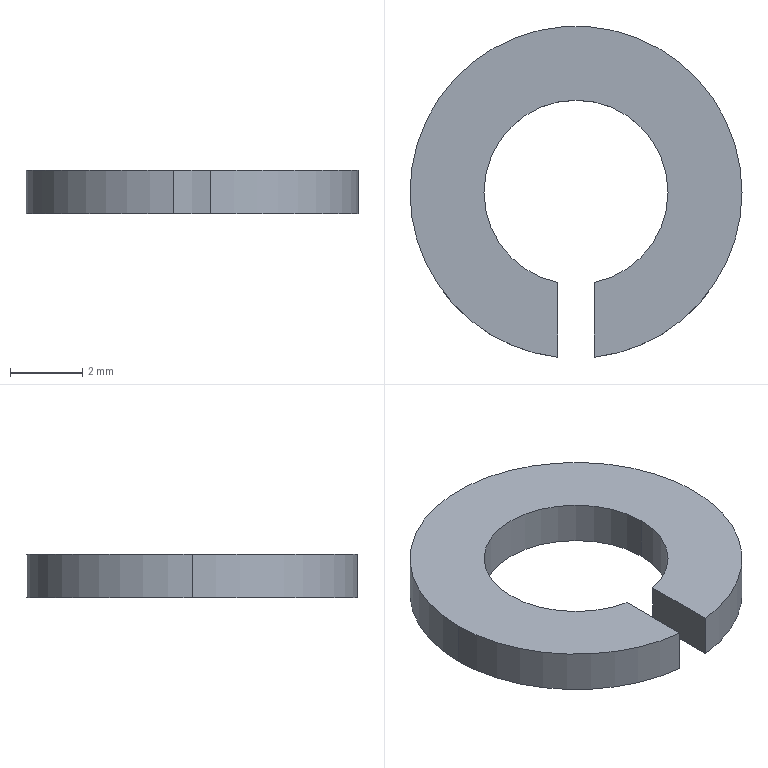Part | NX | features BREP 1 | 1 solid | 10 faces | box 9.2 x 9.173 x 1.2 mm | volume 52.789 mm3 | cylinder 6 | plane 4 | commonest cylinder face diameters 5.1 x3 9.2 x3
STEP:
#1=CARTESIAN_POINT('',(2.55,0.,1.2));
#2=VERTEX_POINT('',#1);
#3=CARTESIAN_POINT('',(0.5,-2.5,1.2));
#4=VERTEX_POINT('',#3);
#5=CARTESIAN_POINT('',(0.,0.,1.2));
#6=DIRECTION('',(0.,0.,-1.));
#7=DIRECTION('',(1.,0.,0.));
#8=AXIS2_PLACEMENT_3D('',#5,#6,#7);
#9=CIRCLE('',#8,2.55);
#10=EDGE_CURVE('',#2,#4,#9,.T.);
#11=ORIENTED_EDGE('',*,*,#10,.F.);
#12=CARTESIAN_POINT('',(2.55,0.,0.));
#13=VERTEX_POINT('',#12);
#14=CARTESIAN_POINT('',(2.55,0.,1.2));
#15=DIRECTION('',(0.,0.,-1.));
#16=VECTOR('',#15,1000.);
#17=LINE('',#14,#16);
#18=EDGE_CURVE('',#2,#13,#17,.T.);
#19=ORIENTED_EDGE('',*,*,#18,.T.);
#20=CARTESIAN_POINT('',(0.5,-2.5,0.));
#21=VERTEX_POINT('',#20);
#22=CARTESIAN_POINT('',(0.,0.,0.));
#23=DIRECTION('',(0.,0.,-1.));
#24=DIRECTION('',(1.,0.,0.));
#25=AXIS2_PLACEMENT_3D('',#22,#23,#24);
#26=CIRCLE('',#25,2.55);
#27=EDGE_CURVE('',#13,#21,#26,.T.);
#28=ORIENTED_EDGE('',*,*,#27,.T.);
#29=CARTESIAN_POINT('',(0.5,-2.5,1.2));
#30=DIRECTION('',(0.,0.,-1.));
#31=VECTOR('',#30,1000.);
#32=LINE('',#29,#31);
#33=EDGE_CURVE('',#4,#21,#32,.T.);
#34=ORIENTED_EDGE('',*,*,#33,.F.);
#35=EDGE_LOOP('',(#11,#19,#28,#34));
#36=FACE_BOUND('',#35,.T.);
#37=CARTESIAN_POINT('',(0.,0.,1.2));
#38=DIRECTION('',(0.,0.,-1.));
#39=DIRECTION('',(-1.,0.,0.));
#40=AXIS2_PLACEMENT_3D('',#37,#38,#39);
#41=CYLINDRICAL_SURFACE('',#40,2.55);
#42=ADVANCED_FACE('',(#36),#41,.F.);
#43=ORIENTED_EDGE('',*,*,#18,.F.);
#44=CARTESIAN_POINT('',(-2.55,0.,1.2));
#45=VERTEX_POINT('',#44);
#46=CARTESIAN_POINT('',(0.,0.,1.2));
#47=DIRECTION('',(0.,0.,-1.));
#48=DIRECTION('',(1.,0.,0.));
#49=AXIS2_PLACEMENT_3D('',#46,#47,#48);
#50=CIRCLE('',#49,2.55);
#51=EDGE_CURVE('',#45,#2,#50,.T.);
#52=ORIENTED_EDGE('',*,*,#51,.F.);
#53=CARTESIAN_POINT('',(-2.55,0.,0.));
#54=VERTEX_POINT('',#53);
#55=CARTESIAN_POINT('',(-2.55,0.,1.2));
#56=DIRECTION('',(0.,0.,-1.));
#57=VECTOR('',#56,1000.);
#58=LINE('',#55,#57);
#59=EDGE_CURVE('',#45,#54,#58,.T.);
#60=ORIENTED_EDGE('',*,*,#59,.T.);
#61=CARTESIAN_POINT('',(0.,0.,0.));
#62=DIRECTION('',(0.,0.,-1.));
#63=DIRECTION('',(1.,0.,0.));
#64=AXIS2_PLACEMENT_3D('',#61,#62,#63);
#65=CIRCLE('',#64,2.55);
#66=EDGE_CURVE('',#54,#13,#65,.T.);
#67=ORIENTED_EDGE('',*,*,#66,.T.);
#68=EDGE_LOOP('',(#43,#52,#60,#67));
#69=FACE_BOUND('',#68,.T.);
#70=CARTESIAN_POINT('',(0.,0.,1.2));
#71=DIRECTION('',(0.,0.,-1.));
#72=DIRECTION('',(-1.,0.,0.));
#73=AXIS2_PLACEMENT_3D('',#70,#71,#72);
#74=CYLINDRICAL_SURFACE('',#73,2.55);
#75=ADVANCED_FACE('',(#69),#74,.F.);
#76=CARTESIAN_POINT('',(4.6,0.,1.2));
#77=VERTEX_POINT('',#76);
#78=CARTESIAN_POINT('',(-4.6,0.,1.2));
#79=VERTEX_POINT('',#78);
#80=CARTESIAN_POINT('',(0.,0.,1.2));
#81=DIRECTION('',(0.,0.,1.));
#82=DIRECTION('',(1.,0.,0.));
#83=AXIS2_PLACEMENT_3D('',#80,#81,#82);
#84=CIRCLE('',#83,4.6);
#85=EDGE_CURVE('',#77,#79,#84,.T.);
#86=ORIENTED_EDGE('',*,*,#85,.F.);
#87=CARTESIAN_POINT('',(4.6,0.,0.));
#88=VERTEX_POINT('',#87);
#89=CARTESIAN_POINT('',(4.6,0.,1.2));
#90=DIRECTION('',(0.,0.,-1.));
#91=VECTOR('',#90,1000.);
#92=LINE('',#89,#91);
#93=EDGE_CURVE('',#77,#88,#92,.T.);
#94=ORIENTED_EDGE('',*,*,#93,.T.);
#95=CARTESIAN_POINT('',(-4.6,0.,0.));
#96=VERTEX_POINT('',#95);
#97=CARTESIAN_POINT('',(0.,0.,0.));
#98=DIRECTION('',(0.,0.,1.));
#99=DIRECTION('',(1.,0.,0.));
#100=AXIS2_PLACEMENT_3D('',#97,#98,#99);
#101=CIRCLE('',#100,4.6);
#102=EDGE_CURVE('',#88,#96,#101,.T.);
#103=ORIENTED_EDGE('',*,*,#102,.T.);
#104=CARTESIAN_POINT('',(-4.6,0.,1.2));
#105=DIRECTION('',(0.,0.,-1.));
#106=VECTOR('',#105,1000.);
#107=LINE('',#104,#106);
#108=EDGE_CURVE('',#79,#96,#107,.T.);
#109=ORIENTED_EDGE('',*,*,#108,.F.);
#110=EDGE_LOOP('',(#86,#94,#103,#109));
#111=FACE_BOUND('',#110,.T.);
#112=CARTESIAN_POINT('',(0.,0.,1.2));
#113=DIRECTION('',(0.,0.,-1.));
#114=DIRECTION('',(-1.,0.,0.));
#115=AXIS2_PLACEMENT_3D('',#112,#113,#114);
#116=CYLINDRICAL_SURFACE('',#115,4.6);
#117=ADVANCED_FACE('',(#111),#116,.T.);
#118=CARTESIAN_POINT('',(-0.5,-4.573,1.2));
#119=VERTEX_POINT('',#118);
#120=CARTESIAN_POINT('',(0.,0.,1.2));
#121=DIRECTION('',(0.,0.,1.));
#122=DIRECTION('',(1.,0.,0.));
#123=AXIS2_PLACEMENT_3D('',#120,#121,#122);
#124=CIRCLE('',#123,4.6);
#125=EDGE_CURVE('',#79,#119,#124,.T.);
#126=ORIENTED_EDGE('',*,*,#125,.F.);
#127=ORIENTED_EDGE('',*,*,#108,.T.);
#128=CARTESIAN_POINT('',(-0.5,-4.573,0.));
#129=VERTEX_POINT('',#128);
#130=CARTESIAN_POINT('',(0.,0.,0.));
#131=DIRECTION('',(0.,0.,1.));
#132=DIRECTION('',(1.,0.,0.));
#133=AXIS2_PLACEMENT_3D('',#130,#131,#132);
#134=CIRCLE('',#133,4.6);
#135=EDGE_CURVE('',#96,#129,#134,.T.);
#136=ORIENTED_EDGE('',*,*,#135,.T.);
#137=CARTESIAN_POINT('',(-0.5,-4.573,1.2));
#138=DIRECTION('',(0.,0.,-1.));
#139=VECTOR('',#138,1000.);
#140=LINE('',#137,#139);
#141=EDGE_CURVE('',#119,#129,#140,.T.);
#142=ORIENTED_EDGE('',*,*,#141,.F.);
#143=EDGE_LOOP('',(#126,#127,#136,#142));
#144=FACE_BOUND('',#143,.T.);
#145=CARTESIAN_POINT('',(0.,0.,1.2));
#146=DIRECTION('',(0.,0.,-1.));
#147=DIRECTION('',(-1.,0.,0.));
#148=AXIS2_PLACEMENT_3D('',#145,#146,#147);
#149=CYLINDRICAL_SURFACE('',#148,4.6);
#150=ADVANCED_FACE('',(#144),#149,.T.);
#151=ORIENTED_EDGE('',*,*,#93,.F.);
#152=CARTESIAN_POINT('',(0.5,-4.573,1.2));
#153=VERTEX_POINT('',#152);
#154=CARTESIAN_POINT('',(0.,0.,1.2));
#155=DIRECTION('',(0.,0.,1.));
#156=DIRECTION('',(1.,0.,0.));
#157=AXIS2_PLACEMENT_3D('',#154,#155,#156);
#158=CIRCLE('',#157,4.6);
#159=EDGE_CURVE('',#153,#77,#158,.T.);
#160=ORIENTED_EDGE('',*,*,#159,.F.);
#161=CARTESIAN_POINT('',(0.5,-4.573,0.));
#162=VERTEX_POINT('',#161);
#163=CARTESIAN_POINT('',(0.5,-4.573,1.2));
#164=DIRECTION('',(0.,0.,-1.));
#165=VECTOR('',#164,1000.);
#166=LINE('',#163,#165);
#167=EDGE_CURVE('',#153,#162,#166,.T.);
#168=ORIENTED_EDGE('',*,*,#167,.T.);
#169=CARTESIAN_POINT('',(0.,0.,0.));
#170=DIRECTION('',(0.,0.,1.));
#171=DIRECTION('',(1.,0.,0.));
#172=AXIS2_PLACEMENT_3D('',#169,#170,#171);
#173=CIRCLE('',#172,4.6);
#174=EDGE_CURVE('',#162,#88,#173,.T.);
#175=ORIENTED_EDGE('',*,*,#174,.T.);
#176=EDGE_LOOP('',(#151,#160,#168,#175));
#177=FACE_BOUND('',#176,.T.);
#178=CARTESIAN_POINT('',(0.,0.,1.2));
#179=DIRECTION('',(0.,0.,-1.));
#180=DIRECTION('',(-1.,0.,0.));
#181=AXIS2_PLACEMENT_3D('',#178,#179,#180);
#182=CYLINDRICAL_SURFACE('',#181,4.6);
#183=ADVANCED_FACE('',(#177),#182,.T.);
#184=CARTESIAN_POINT('',(-0.5,-2.5,0.));
#185=VERTEX_POINT('',#184);
#186=CARTESIAN_POINT('',(-0.5,-2.5,0.));
#187=DIRECTION('',(0.,1.,0.));
#188=VECTOR('',#187,1000.);
#189=LINE('',#186,#188);
#190=EDGE_CURVE('',#129,#185,#189,.T.);
#191=ORIENTED_EDGE('',*,*,#190,.T.);
#192=CARTESIAN_POINT('',(-0.5,-2.5,1.2));
#193=VERTEX_POINT('',#192);
#194=CARTESIAN_POINT('',(-0.5,-2.5,1.2));
#195=DIRECTION('',(0.,0.,-1.));
#196=VECTOR('',#195,1000.);
#197=LINE('',#194,#196);
#198=EDGE_CURVE('',#193,#185,#197,.T.);
#199=ORIENTED_EDGE('',*,*,#198,.F.);
#200=CARTESIAN_POINT('',(-0.5,-2.5,1.2));
#201=DIRECTION('',(0.,1.,0.));
#202=VECTOR('',#201,1000.);
#203=LINE('',#200,#202);
#204=EDGE_CURVE('',#119,#193,#203,.T.);
#205=ORIENTED_EDGE('',*,*,#204,.F.);
#206=ORIENTED_EDGE('',*,*,#141,.T.);
#207=EDGE_LOOP('',(#191,#199,#205,#206));
#208=FACE_BOUND('',#207,.T.);
#209=CARTESIAN_POINT('',(-0.5,-2.5,1.2));
#210=DIRECTION('',(-1.,0.,0.));
#211=DIRECTION('',(0.,0.,1.));
#212=AXIS2_PLACEMENT_3D('',#209,#210,#211);
#213=PLANE('',#212);
#214=ADVANCED_FACE('',(#208),#213,.F.);
#215=ORIENTED_EDGE('',*,*,#59,.F.);
#216=CARTESIAN_POINT('',(0.,0.,1.2));
#217=DIRECTION('',(0.,0.,-1.));
#218=DIRECTION('',(1.,0.,0.));
#219=AXIS2_PLACEMENT_3D('',#216,#217,#218);
#220=CIRCLE('',#219,2.55);
#221=EDGE_CURVE('',#193,#45,#220,.T.);
#222=ORIENTED_EDGE('',*,*,#221,.F.);
#223=ORIENTED_EDGE('',*,*,#198,.T.);
#224=CARTESIAN_POINT('',(0.,0.,0.));
#225=DIRECTION('',(0.,0.,-1.));
#226=DIRECTION('',(1.,0.,0.));
#227=AXIS2_PLACEMENT_3D('',#224,#225,#226);
#228=CIRCLE('',#227,2.55);
#229=EDGE_CURVE('',#185,#54,#228,.T.);
#230=ORIENTED_EDGE('',*,*,#229,.T.);
#231=EDGE_LOOP('',(#215,#222,#223,#230));
#232=FACE_BOUND('',#231,.T.);
#233=CARTESIAN_POINT('',(0.,0.,1.2));
#234=DIRECTION('',(0.,0.,-1.));
#235=DIRECTION('',(-1.,0.,0.));
#236=AXIS2_PLACEMENT_3D('',#233,#234,#235);
#237=CYLINDRICAL_SURFACE('',#236,2.55);
#238=ADVANCED_FACE('',(#232),#237,.F.);
#239=CARTESIAN_POINT('',(0.5,-2.5,0.));
#240=DIRECTION('',(0.,-1.,0.));
#241=VECTOR('',#240,1000.);
#242=LINE('',#239,#241);
#243=EDGE_CURVE('',#21,#162,#242,.T.);
#244=ORIENTED_EDGE('',*,*,#243,.T.);
#245=ORIENTED_EDGE('',*,*,#167,.F.);
#246=CARTESIAN_POINT('',(0.5,-2.5,1.2));
#247=DIRECTION('',(0.,-1.,0.));
#248=VECTOR('',#247,1000.);
#249=LINE('',#246,#248);
#250=EDGE_CURVE('',#4,#153,#249,.T.);
#251=ORIENTED_EDGE('',*,*,#250,.F.);
#252=ORIENTED_EDGE('',*,*,#33,.T.);
#253=EDGE_LOOP('',(#244,#245,#251,#252));
#254=FACE_BOUND('',#253,.T.);
#255=CARTESIAN_POINT('',(0.5,-2.5,1.2));
#256=DIRECTION('',(1.,0.,0.));
#257=DIRECTION('',(0.,1.,0.));
#258=AXIS2_PLACEMENT_3D('',#255,#256,#257);
#259=PLANE('',#258);
#260=ADVANCED_FACE('',(#254),#259,.F.);
#261=ORIENTED_EDGE('',*,*,#159,.T.);
#262=ORIENTED_EDGE('',*,*,#85,.T.);
#263=ORIENTED_EDGE('',*,*,#125,.T.);
#264=ORIENTED_EDGE('',*,*,#204,.T.);
#265=ORIENTED_EDGE('',*,*,#221,.T.);
#266=ORIENTED_EDGE('',*,*,#51,.T.);
#267=ORIENTED_EDGE('',*,*,#10,.T.);
#268=ORIENTED_EDGE('',*,*,#250,.T.);
#269=EDGE_LOOP('',(#261,#262,#263,#264,#265,#266,#267,#268));
#270=FACE_BOUND('',#269,.T.);
#271=CARTESIAN_POINT('',(0.,0.,1.2));
#272=DIRECTION('',(0.,0.,1.));
#273=DIRECTION('',(1.,0.,0.));
#274=AXIS2_PLACEMENT_3D('',#271,#272,#273);
#275=PLANE('',#274);
#276=ADVANCED_FACE('',(#270),#275,.T.);
#277=ORIENTED_EDGE('',*,*,#174,.F.);
#278=ORIENTED_EDGE('',*,*,#243,.F.);
#279=ORIENTED_EDGE('',*,*,#27,.F.);
#280=ORIENTED_EDGE('',*,*,#66,.F.);
#281=ORIENTED_EDGE('',*,*,#229,.F.);
#282=ORIENTED_EDGE('',*,*,#190,.F.);
#283=ORIENTED_EDGE('',*,*,#135,.F.);
#284=ORIENTED_EDGE('',*,*,#102,.F.);
#285=EDGE_LOOP('',(#277,#278,#279,#280,#281,#282,#283,#284));
#286=FACE_BOUND('',#285,.T.);
#287=CARTESIAN_POINT('',(0.,0.,0.));
#288=DIRECTION('',(0.,0.,1.));
#289=DIRECTION('',(1.,0.,0.));
#290=AXIS2_PLACEMENT_3D('',#287,#288,#289);
#291=PLANE('',#290);
#292=ADVANCED_FACE('',(#286),#291,.F.);
#293=CLOSED_SHELL('',(#42,#75,#117,#150,#183,#214,#238,#260,#276,#292));
#294=MANIFOLD_SOLID_BREP('',#293);
#295=(LENGTH_UNIT()NAMED_UNIT(*)SI_UNIT(.MILLI.,.METRE.));
#296=UNCERTAINTY_MEASURE_WITH_UNIT(LENGTH_MEASURE(0.00001),#295,'','');
#297=(NAMED_UNIT(*)PLANE_ANGLE_UNIT()SI_UNIT($,.RADIAN.));
#298=(NAMED_UNIT(*)SI_UNIT($,.STERADIAN.)SOLID_ANGLE_UNIT());
#299=(GEOMETRIC_REPRESENTATION_CONTEXT(3)GLOBAL_UNCERTAINTY_ASSIGNED_CONTEXT((#296))GLOBAL_UNIT_ASSIGNED_CONTEXT((#295,#297,#298))REPRESENTATION_CONTEXT('',''));
#300=ADVANCED_BREP_SHAPE_REPRESENTATION('',(#294),#299);